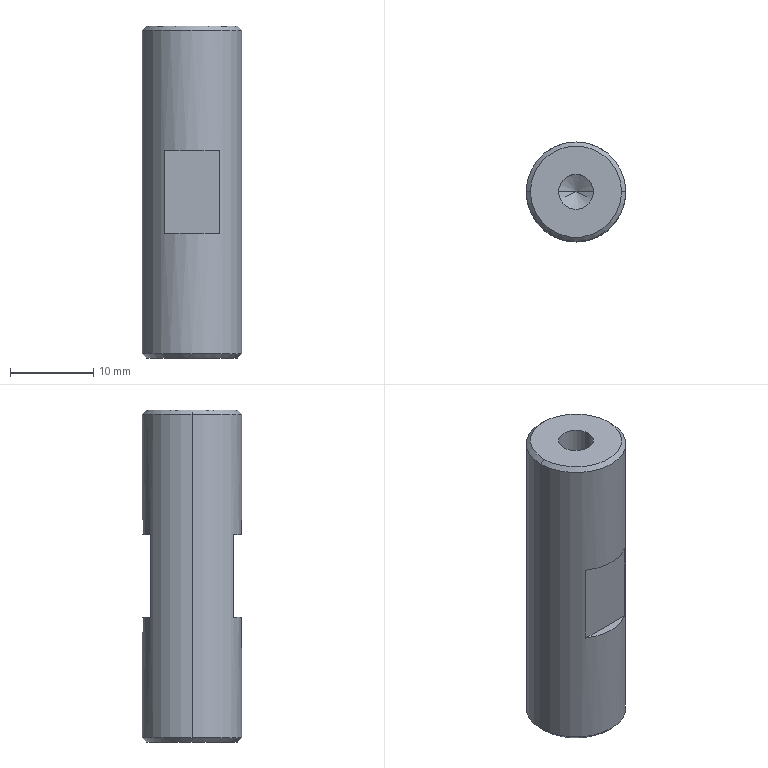Part | STEP file | QA-FC07 | 1 solid | 22 faces | box 12 x 12 x 40 mm | volume 4081 mm3 | cone 8 | plane 8 | cylinder 6 | commonest cylinder face diameters 4.2 x4 12 x2
STEP:
#1=CARTESIAN_POINT('',(0.,0.,0.));
#2=DIRECTION('',(0.,0.,1.));
#3=DIRECTION('',(1.,0.,0.));
#4=AXIS2_PLACEMENT_3D('',#1,#2,#3);
#5=CARTESIAN_POINT('',(5.5,0.,40.));
#6=VERTEX_POINT('',#5);
#7=CARTESIAN_POINT('',(-5.5,0.,40.));
#8=VERTEX_POINT('',#7);
#9=CARTESIAN_POINT('',(0.,0.,40.));
#10=DIRECTION('',(0.,0.,1.));
#11=DIRECTION('',(1.,0.,0.));
#12=AXIS2_PLACEMENT_3D('',#9,#10,#11);
#13=CIRCLE('',#12,5.5);
#14=CARTESIAN_POINT('',(0.,0.,40.));
#15=DIRECTION('',(0.,0.,-1.));
#16=DIRECTION('',(-1.,0.,0.));
#17=AXIS2_PLACEMENT_3D('',#14,#15,#16);
#18=CONICAL_SURFACE('',#17,5.5,0.7854);
#19=CARTESIAN_POINT('',(3.142,0.));
#20=DIRECTION('',(-1.,0.));
#21=VECTOR('',#20,1.);
#22=LINE('',#19,#21);
#23=(GEOMETRIC_REPRESENTATION_CONTEXT(2)PARAMETRIC_REPRESENTATION_CONTEXT()REPRESENTATION_CONTEXT('',''));
#24=DEFINITIONAL_REPRESENTATION('',(#22),#23);
#25=PCURVE('',#18,#24);
#26=CARTESIAN_POINT('',(0.,0.,40.));
#27=DIRECTION('',(0.,0.,1.));
#28=DIRECTION('',(1.,0.,0.));
#29=AXIS2_PLACEMENT_3D('',#26,#27,#28);
#30=PLANE('',#29);
#31=CARTESIAN_POINT('',(0.,0.));
#32=DIRECTION('',(1.,0.));
#33=AXIS2_PLACEMENT_2D('',#31,#32);
#34=CIRCLE('',#33,5.5);
#35=(GEOMETRIC_REPRESENTATION_CONTEXT(2)PARAMETRIC_REPRESENTATION_CONTEXT()REPRESENTATION_CONTEXT('',''));
#36=DEFINITIONAL_REPRESENTATION('',(#34),#35);
#37=PCURVE('',#30,#36);
#38=SURFACE_CURVE('',#13,(#25,#37),.PCURVE_S1.);
#39=EDGE_CURVE('',#6,#8,#38,.T.);
#40=ORIENTED_EDGE('',*,*,#39,.F.);
#41=CARTESIAN_POINT('',(6.,0.,39.5));
#42=VERTEX_POINT('',#41);
#43=CARTESIAN_POINT('',(5.5,0.,40.));
#44=DIRECTION('',(0.7071,0.,-0.7071));
#45=VECTOR('',#44,1.);
#46=LINE('',#43,#45);
#47=CARTESIAN_POINT('',(3.142,0.));
#48=DIRECTION('',(0.,1.));
#49=VECTOR('',#48,1.);
#50=LINE('',#47,#49);
#51=(GEOMETRIC_REPRESENTATION_CONTEXT(2)PARAMETRIC_REPRESENTATION_CONTEXT()REPRESENTATION_CONTEXT('',''));
#52=DEFINITIONAL_REPRESENTATION('',(#50),#51);
#53=PCURVE('',#18,#52);
#54=CARTESIAN_POINT('',(0.,0.,40.));
#55=DIRECTION('',(0.,0.,-1.));
#56=DIRECTION('',(-1.,0.,0.));
#57=AXIS2_PLACEMENT_3D('',#54,#55,#56);
#58=CONICAL_SURFACE('',#57,5.5,0.7854);
#59=CARTESIAN_POINT('',(3.142,0.));
#60=DIRECTION('',(0.,1.));
#61=VECTOR('',#60,1.);
#62=LINE('',#59,#61);
#63=(GEOMETRIC_REPRESENTATION_CONTEXT(2)PARAMETRIC_REPRESENTATION_CONTEXT()REPRESENTATION_CONTEXT('',''));
#64=DEFINITIONAL_REPRESENTATION('',(#62),#63);
#65=PCURVE('',#58,#64);
#66=SURFACE_CURVE('',#46,(#53,#65),.PCURVE_S1.);
#67=EDGE_CURVE('',#6,#42,#66,.T.);
#68=ORIENTED_EDGE('',*,*,#67,.T.);
#69=CARTESIAN_POINT('',(-6.,0.,39.5));
#70=VERTEX_POINT('',#69);
#71=CARTESIAN_POINT('',(0.,0.,39.5));
#72=DIRECTION('',(0.,0.,-1.));
#73=DIRECTION('',(1.,0.,0.));
#74=AXIS2_PLACEMENT_3D('',#71,#72,#73);
#75=CIRCLE('',#74,6.);
#76=CARTESIAN_POINT('',(-3.142,0.5));
#77=DIRECTION('',(1.,0.));
#78=VECTOR('',#77,1.);
#79=LINE('',#76,#78);
#80=(GEOMETRIC_REPRESENTATION_CONTEXT(2)PARAMETRIC_REPRESENTATION_CONTEXT()REPRESENTATION_CONTEXT('',''));
#81=DEFINITIONAL_REPRESENTATION('',(#79),#80);
#82=PCURVE('',#18,#81);
#83=CARTESIAN_POINT('',(0.,0.,40.));
#84=DIRECTION('',(0.,0.,-1.));
#85=DIRECTION('',(-1.,0.,0.));
#86=AXIS2_PLACEMENT_3D('',#83,#84,#85);
#87=CYLINDRICAL_SURFACE('',#86,6.);
#88=CARTESIAN_POINT('',(-3.142,0.5));
#89=DIRECTION('',(1.,0.));
#90=VECTOR('',#89,1.);
#91=LINE('',#88,#90);
#92=(GEOMETRIC_REPRESENTATION_CONTEXT(2)PARAMETRIC_REPRESENTATION_CONTEXT()REPRESENTATION_CONTEXT('',''));
#93=DEFINITIONAL_REPRESENTATION('',(#91),#92);
#94=PCURVE('',#87,#93);
#95=SURFACE_CURVE('',#75,(#82,#94),.PCURVE_S1.);
#96=EDGE_CURVE('',#70,#42,#95,.T.);
#97=ORIENTED_EDGE('',*,*,#96,.F.);
#98=CARTESIAN_POINT('',(-5.5,0.,40.));
#99=DIRECTION('',(-0.7071,0.,-0.7071));
#100=VECTOR('',#99,1.);
#101=LINE('',#98,#100);
#102=CARTESIAN_POINT('',(0.,0.));
#103=DIRECTION('',(0.,1.));
#104=VECTOR('',#103,1.);
#105=LINE('',#102,#104);
#106=(GEOMETRIC_REPRESENTATION_CONTEXT(2)PARAMETRIC_REPRESENTATION_CONTEXT()REPRESENTATION_CONTEXT('',''));
#107=DEFINITIONAL_REPRESENTATION('',(#105),#106);
#108=PCURVE('',#18,#107);
#109=CARTESIAN_POINT('',(6.283,0.));
#110=DIRECTION('',(0.,1.));
#111=VECTOR('',#110,1.);
#112=LINE('',#109,#111);
#113=(GEOMETRIC_REPRESENTATION_CONTEXT(2)PARAMETRIC_REPRESENTATION_CONTEXT()REPRESENTATION_CONTEXT('',''));
#114=DEFINITIONAL_REPRESENTATION('',(#112),#113);
#115=PCURVE('',#58,#114);
#116=SURFACE_CURVE('',#101,(#108,#115),.PCURVE_S1.);
#117=EDGE_CURVE('',#8,#70,#116,.T.);
#118=ORIENTED_EDGE('',*,*,#117,.F.);
#119=EDGE_LOOP('',(#40,#68,#97,#118));
#120=FACE_BOUND('',#119,.T.);
#121=ADVANCED_FACE('',(#120),#18,.T.);
#122=CARTESIAN_POINT('',(-5.5,0.,0.));
#123=VERTEX_POINT('',#122);
#124=CARTESIAN_POINT('',(5.5,0.,0.));
#125=VERTEX_POINT('',#124);
#126=CARTESIAN_POINT('',(0.,0.,0.));
#127=DIRECTION('',(0.,0.,-1.));
#128=DIRECTION('',(1.,0.,0.));
#129=AXIS2_PLACEMENT_3D('',#126,#127,#128);
#130=CIRCLE('',#129,5.5);
#131=CARTESIAN_POINT('',(0.,0.,0.5));
#132=DIRECTION('',(0.,0.,1.));
#133=DIRECTION('',(1.,0.,0.));
#134=AXIS2_PLACEMENT_3D('',#131,#132,#133);
#135=CONICAL_SURFACE('',#134,6.,0.7854);
#136=CARTESIAN_POINT('',(6.283,-0.5));
#137=DIRECTION('',(-1.,0.));
#138=VECTOR('',#137,1.);
#139=LINE('',#136,#138);
#140=(GEOMETRIC_REPRESENTATION_CONTEXT(2)PARAMETRIC_REPRESENTATION_CONTEXT()REPRESENTATION_CONTEXT('',''));
#141=DEFINITIONAL_REPRESENTATION('',(#139),#140);
#142=PCURVE('',#135,#141);
#143=CARTESIAN_POINT('',(0.,0.,0.));
#144=DIRECTION('',(0.,0.,1.));
#145=DIRECTION('',(1.,0.,0.));
#146=AXIS2_PLACEMENT_3D('',#143,#144,#145);
#147=PLANE('',#146);
#148=CARTESIAN_POINT('',(5.5,0.));
#149=CARTESIAN_POINT('',(5.5,-9.526));
#150=CARTESIAN_POINT('',(-2.75,-4.763));
#151=CARTESIAN_POINT('',(-11.,0.));
#152=CARTESIAN_POINT('',(-2.75,4.763));
#153=CARTESIAN_POINT('',(5.5,9.526));
#154=CARTESIAN_POINT('',(5.5,0.));
#155=(BOUNDED_CURVE()B_SPLINE_CURVE(2,(#148,#149,#150,#151,#152,#153,#154),.UNSPECIFIED.,.T.,.F.)B_SPLINE_CURVE_WITH_KNOTS((1,2,2,2,2,1),(-2.094,0.,2.094,4.189,6.283,8.378),.UNSPECIFIED.)CURVE()GEOMETRIC_REPRESENTATION_ITEM()RATIONAL_B_SPLINE_CURVE((1.,0.5,1.,0.5,1.,0.5,1.))REPRESENTATION_ITEM(''));
#156=(GEOMETRIC_REPRESENTATION_CONTEXT(2)PARAMETRIC_REPRESENTATION_CONTEXT()REPRESENTATION_CONTEXT('',''));
#157=DEFINITIONAL_REPRESENTATION('',(#155),#156);
#158=PCURVE('',#147,#157);
#159=SURFACE_CURVE('',#130,(#142,#158),.PCURVE_S1.);
#160=EDGE_CURVE('',#123,#125,#159,.T.);
#161=ORIENTED_EDGE('',*,*,#160,.F.);
#162=CARTESIAN_POINT('',(-6.,0.,0.5));
#163=VERTEX_POINT('',#162);
#164=CARTESIAN_POINT('',(-6.,0.,0.5));
#165=DIRECTION('',(-0.7071,0.,0.7071));
#166=VECTOR('',#165,1.);
#167=LINE('',#164,#166);
#168=CARTESIAN_POINT('',(3.142,0.));
#169=DIRECTION('',(0.,1.));
#170=VECTOR('',#169,1.);
#171=LINE('',#168,#170);
#172=(GEOMETRIC_REPRESENTATION_CONTEXT(2)PARAMETRIC_REPRESENTATION_CONTEXT()REPRESENTATION_CONTEXT('',''));
#173=DEFINITIONAL_REPRESENTATION('',(#171),#172);
#174=PCURVE('',#135,#173);
#175=CARTESIAN_POINT('',(0.,0.,0.5));
#176=DIRECTION('',(0.,0.,1.));
#177=DIRECTION('',(1.,0.,0.));
#178=AXIS2_PLACEMENT_3D('',#175,#176,#177);
#179=CONICAL_SURFACE('',#178,6.,0.7854);
#180=CARTESIAN_POINT('',(3.142,0.));
#181=DIRECTION('',(0.,1.));
#182=VECTOR('',#181,1.);
#183=LINE('',#180,#182);
#184=(GEOMETRIC_REPRESENTATION_CONTEXT(2)PARAMETRIC_REPRESENTATION_CONTEXT()REPRESENTATION_CONTEXT('',''));
#185=DEFINITIONAL_REPRESENTATION('',(#183),#184);
#186=PCURVE('',#179,#185);
#187=SURFACE_CURVE('',#167,(#174,#186),.PCURVE_S1.);
#188=EDGE_CURVE('',#123,#163,#187,.T.);
#189=ORIENTED_EDGE('',*,*,#188,.T.);
#190=CARTESIAN_POINT('',(6.,0.,0.5));
#191=VERTEX_POINT('',#190);
#192=CARTESIAN_POINT('',(0.,0.,0.5));
#193=DIRECTION('',(0.,0.,1.));
#194=DIRECTION('',(1.,0.,0.));
#195=AXIS2_PLACEMENT_3D('',#192,#193,#194);
#196=CIRCLE('',#195,6.);
#197=CARTESIAN_POINT('',(0.,0.));
#198=DIRECTION('',(1.,0.));
#199=VECTOR('',#198,1.);
#200=LINE('',#197,#199);
#201=(GEOMETRIC_REPRESENTATION_CONTEXT(2)PARAMETRIC_REPRESENTATION_CONTEXT()REPRESENTATION_CONTEXT('',''));
#202=DEFINITIONAL_REPRESENTATION('',(#200),#201);
#203=PCURVE('',#135,#202);
#204=CARTESIAN_POINT('',(3.142,39.5));
#205=DIRECTION('',(-1.,0.));
#206=VECTOR('',#205,1.);
#207=LINE('',#204,#206);
#208=(GEOMETRIC_REPRESENTATION_CONTEXT(2)PARAMETRIC_REPRESENTATION_CONTEXT()REPRESENTATION_CONTEXT('',''));
#209=DEFINITIONAL_REPRESENTATION('',(#207),#208);
#210=PCURVE('',#87,#209);
#211=SURFACE_CURVE('',#196,(#203,#210),.PCURVE_S1.);
#212=EDGE_CURVE('',#191,#163,#211,.T.);
#213=ORIENTED_EDGE('',*,*,#212,.F.);
#214=CARTESIAN_POINT('',(6.,0.,0.5));
#215=DIRECTION('',(0.7071,0.,0.7071));
#216=VECTOR('',#215,1.);
#217=LINE('',#214,#216);
#218=CARTESIAN_POINT('',(0.,0.));
#219=DIRECTION('',(0.,1.));
#220=VECTOR('',#219,1.);
#221=LINE('',#218,#220);
#222=(GEOMETRIC_REPRESENTATION_CONTEXT(2)PARAMETRIC_REPRESENTATION_CONTEXT()REPRESENTATION_CONTEXT('',''));
#223=DEFINITIONAL_REPRESENTATION('',(#221),#222);
#224=PCURVE('',#135,#223);
#225=CARTESIAN_POINT('',(6.283,0.));
#226=DIRECTION('',(0.,1.));
#227=VECTOR('',#226,1.);
#228=LINE('',#225,#227);
#229=(GEOMETRIC_REPRESENTATION_CONTEXT(2)PARAMETRIC_REPRESENTATION_CONTEXT()REPRESENTATION_CONTEXT('',''));
#230=DEFINITIONAL_REPRESENTATION('',(#228),#229);
#231=PCURVE('',#179,#230);
#232=SURFACE_CURVE('',#217,(#224,#231),.PCURVE_S1.);
#233=EDGE_CURVE('',#125,#191,#232,.T.);
#234=ORIENTED_EDGE('',*,*,#233,.F.);
#235=EDGE_LOOP('',(#161,#189,#213,#234));
#236=FACE_BOUND('',#235,.T.);
#237=ADVANCED_FACE('',(#236),#135,.T.);
#238=CARTESIAN_POINT('',(-2.1,0.,12.));
#239=VERTEX_POINT('',#238);
#240=CARTESIAN_POINT('',(-2.1,0.,0.));
#241=VERTEX_POINT('',#240);
#242=CARTESIAN_POINT('',(-2.1,0.,0.));
#243=DIRECTION('',(0.,0.,-1.));
#244=VECTOR('',#243,1.);
#245=LINE('',#242,#244);
#246=CARTESIAN_POINT('',(0.,0.,0.));
#247=DIRECTION('',(0.,0.,-1.));
#248=DIRECTION('',(-1.,0.,0.));
#249=AXIS2_PLACEMENT_3D('',#246,#247,#248);
#250=CYLINDRICAL_SURFACE('',#249,2.1);
#251=CARTESIAN_POINT('',(6.283,0.));
#252=DIRECTION('',(0.,1.));
#253=VECTOR('',#252,1.);
#254=LINE('',#251,#253);
#255=(GEOMETRIC_REPRESENTATION_CONTEXT(2)PARAMETRIC_REPRESENTATION_CONTEXT()REPRESENTATION_CONTEXT('',''));
#256=DEFINITIONAL_REPRESENTATION('',(#254),#255);
#257=PCURVE('',#250,#256);
#258=CARTESIAN_POINT('',(0.,0.,0.));
#259=DIRECTION('',(0.,0.,-1.));
#260=DIRECTION('',(-1.,0.,0.));
#261=AXIS2_PLACEMENT_3D('',#258,#259,#260);
#262=CYLINDRICAL_SURFACE('',#261,2.1);
#263=CARTESIAN_POINT('',(0.,0.));
#264=DIRECTION('',(0.,1.));
#265=VECTOR('',#264,1.);
#266=LINE('',#263,#265);
#267=(GEOMETRIC_REPRESENTATION_CONTEXT(2)PARAMETRIC_REPRESENTATION_CONTEXT()REPRESENTATION_CONTEXT('',''));
#268=DEFINITIONAL_REPRESENTATION('',(#266),#267);
#269=PCURVE('',#262,#268);
#270=SURFACE_CURVE('',#245,(#257,#269),.PCURVE_S1.);
#271=EDGE_CURVE('',#239,#241,#270,.T.);
#272=ORIENTED_EDGE('',*,*,#271,.T.);
#273=CARTESIAN_POINT('',(2.1,0.,0.));
#274=VERTEX_POINT('',#273);
#275=CARTESIAN_POINT('',(0.,0.,0.));
#276=DIRECTION('',(0.,0.,-1.));
#277=DIRECTION('',(-1.,0.,0.));
#278=AXIS2_PLACEMENT_3D('',#275,#276,#277);
#279=CIRCLE('',#278,2.1);
#280=CARTESIAN_POINT('',(0.,0.));
#281=DIRECTION('',(1.,0.));
#282=VECTOR('',#281,1.);
#283=LINE('',#280,#282);
#284=(GEOMETRIC_REPRESENTATION_CONTEXT(2)PARAMETRIC_REPRESENTATION_CONTEXT()REPRESENTATION_CONTEXT('',''));
#285=DEFINITIONAL_REPRESENTATION('',(#283),#284);
#286=PCURVE('',#250,#285);
#287=CARTESIAN_POINT('',(-2.1,0.));
#288=CARTESIAN_POINT('',(-2.1,3.637));
#289=CARTESIAN_POINT('',(1.05,1.819));
#290=CARTESIAN_POINT('',(4.2,0.));
#291=CARTESIAN_POINT('',(1.05,-1.819));
#292=CARTESIAN_POINT('',(-2.1,-3.637));
#293=CARTESIAN_POINT('',(-2.1,0.));
#294=(BOUNDED_CURVE()B_SPLINE_CURVE(2,(#287,#288,#289,#290,#291,#292,#293),.UNSPECIFIED.,.T.,.F.)B_SPLINE_CURVE_WITH_KNOTS((1,2,2,2,2,1),(-2.094,0.,2.094,4.189,6.283,8.378),.UNSPECIFIED.)CURVE()GEOMETRIC_REPRESENTATION_ITEM()RATIONAL_B_SPLINE_CURVE((1.,0.5,1.,0.5,1.,0.5,1.))REPRESENTATION_ITEM(''));
#295=(GEOMETRIC_REPRESENTATION_CONTEXT(2)PARAMETRIC_REPRESENTATION_CONTEXT()REPRESENTATION_CONTEXT('',''));
#296=DEFINITIONAL_REPRESENTATION('',(#294),#295);
#297=PCURVE('',#147,#296);
#298=SURFACE_CURVE('',#279,(#286,#297),.PCURVE_S1.);
#299=EDGE_CURVE('',#274,#241,#298,.T.);
#300=ORIENTED_EDGE('',*,*,#299,.F.);
#301=CARTESIAN_POINT('',(2.1,0.,12.));
#302=VERTEX_POINT('',#301);
#303=CARTESIAN_POINT('',(2.1,0.,0.));
#304=DIRECTION('',(0.,0.,-1.));
#305=VECTOR('',#304,1.);
#306=LINE('',#303,#305);
#307=CARTESIAN_POINT('',(3.142,0.));
#308=DIRECTION('',(0.,1.));
#309=VECTOR('',#308,1.);
#310=LINE('',#307,#309);
#311=(GEOMETRIC_REPRESENTATION_CONTEXT(2)PARAMETRIC_REPRESENTATION_CONTEXT()REPRESENTATION_CONTEXT('',''));
#312=DEFINITIONAL_REPRESENTATION('',(#310),#311);
#313=PCURVE('',#250,#312);
#314=CARTESIAN_POINT('',(3.142,0.));
#315=DIRECTION('',(0.,1.));
#316=VECTOR('',#315,1.);
#317=LINE('',#314,#316);
#318=(GEOMETRIC_REPRESENTATION_CONTEXT(2)PARAMETRIC_REPRESENTATION_CONTEXT()REPRESENTATION_CONTEXT('',''));
#319=DEFINITIONAL_REPRESENTATION('',(#317),#318);
#320=PCURVE('',#262,#319);
#321=SURFACE_CURVE('',#306,(#313,#320),.PCURVE_S1.);
#322=EDGE_CURVE('',#302,#274,#321,.T.);
#323=ORIENTED_EDGE('',*,*,#322,.F.);
#324=CARTESIAN_POINT('',(0.,0.,12.));
#325=DIRECTION('',(0.,0.,-1.));
#326=DIRECTION('',(-1.,0.,0.));
#327=AXIS2_PLACEMENT_3D('',#324,#325,#326);
#328=CIRCLE('',#327,2.1);
#329=CARTESIAN_POINT('',(0.,-12.));
#330=DIRECTION('',(1.,0.));
#331=VECTOR('',#330,1.);
#332=LINE('',#329,#331);
#333=(GEOMETRIC_REPRESENTATION_CONTEXT(2)PARAMETRIC_REPRESENTATION_CONTEXT()REPRESENTATION_CONTEXT('',''));
#334=DEFINITIONAL_REPRESENTATION('',(#332),#333);
#335=PCURVE('',#250,#334);
#336=CARTESIAN_POINT('',(0.,0.,12.));
#337=DIRECTION('',(0.,0.,-1.));
#338=DIRECTION('',(-1.,0.,0.));
#339=AXIS2_PLACEMENT_3D('',#336,#337,#338);
#340=CONICAL_SURFACE('',#339,2.1,1.03);
#341=CARTESIAN_POINT('',(0.,0.));
#342=DIRECTION('',(1.,0.));
#343=VECTOR('',#342,1.);
#344=LINE('',#341,#343);
#345=(GEOMETRIC_REPRESENTATION_CONTEXT(2)PARAMETRIC_REPRESENTATION_CONTEXT()REPRESENTATION_CONTEXT('',''));
#346=DEFINITIONAL_REPRESENTATION('',(#344),#345);
#347=PCURVE('',#340,#346);
#348=SURFACE_CURVE('',#328,(#335,#347),.PCURVE_S1.);
#349=EDGE_CURVE('',#302,#239,#348,.T.);
#350=ORIENTED_EDGE('',*,*,#349,.T.);
#351=EDGE_LOOP('',(#272,#300,#323,#350));
#352=FACE_BOUND('',#351,.F.);
#353=ADVANCED_FACE('',(#352),#250,.F.);
#354=ORIENTED_EDGE('',*,*,#349,.F.);
#355=CARTESIAN_POINT('',(0.,0.,13.262));
#356=VERTEX_POINT('',#355);
#357=CARTESIAN_POINT('',(2.1,0.,12.));
#358=DIRECTION('',(0.8572,0.,-0.515));
#359=VECTOR('',#358,1.);
#360=LINE('',#357,#359);
#361=CARTESIAN_POINT('',(3.142,0.));
#362=DIRECTION('',(0.,1.));
#363=VECTOR('',#362,1.);
#364=LINE('',#361,#363);
#365=(GEOMETRIC_REPRESENTATION_CONTEXT(2)PARAMETRIC_REPRESENTATION_CONTEXT()REPRESENTATION_CONTEXT('',''));
#366=DEFINITIONAL_REPRESENTATION('',(#364),#365);
#367=PCURVE('',#340,#366);
#368=CARTESIAN_POINT('',(0.,0.,12.));
#369=DIRECTION('',(0.,0.,-1.));
#370=DIRECTION('',(-1.,0.,0.));
#371=AXIS2_PLACEMENT_3D('',#368,#369,#370);
#372=CONICAL_SURFACE('',#371,2.1,1.03);
#373=CARTESIAN_POINT('',(3.142,0.));
#374=DIRECTION('',(0.,1.));
#375=VECTOR('',#374,1.);
#376=LINE('',#373,#375);
#377=(GEOMETRIC_REPRESENTATION_CONTEXT(2)PARAMETRIC_REPRESENTATION_CONTEXT()REPRESENTATION_CONTEXT('',''));
#378=DEFINITIONAL_REPRESENTATION('',(#376),#377);
#379=PCURVE('',#372,#378);
#380=SURFACE_CURVE('',#360,(#367,#379),.PCURVE_S1.);
#381=EDGE_CURVE('',#356,#302,#380,.T.);
#382=ORIENTED_EDGE('',*,*,#381,.F.);
#383=CARTESIAN_POINT('',(-2.1,0.,12.));
#384=DIRECTION('',(-0.8572,0.,-0.515));
#385=VECTOR('',#384,1.);
#386=LINE('',#383,#385);
#387=CARTESIAN_POINT('',(6.283,0.));
#388=DIRECTION('',(0.,1.));
#389=VECTOR('',#388,1.);
#390=LINE('',#387,#389);
#391=(GEOMETRIC_REPRESENTATION_CONTEXT(2)PARAMETRIC_REPRESENTATION_CONTEXT()REPRESENTATION_CONTEXT('',''));
#392=DEFINITIONAL_REPRESENTATION('',(#390),#391);
#393=PCURVE('',#340,#392);
#394=CARTESIAN_POINT('',(0.,0.));
#395=DIRECTION('',(0.,1.));
#396=VECTOR('',#395,1.);
#397=LINE('',#394,#396);
#398=(GEOMETRIC_REPRESENTATION_CONTEXT(2)PARAMETRIC_REPRESENTATION_CONTEXT()REPRESENTATION_CONTEXT('',''));
#399=DEFINITIONAL_REPRESENTATION('',(#397),#398);
#400=PCURVE('',#372,#399);
#401=SURFACE_CURVE('',#386,(#393,#400),.PCURVE_S1.);
#402=EDGE_CURVE('',#356,#239,#401,.T.);
#403=ORIENTED_EDGE('',*,*,#402,.T.);
#404=EDGE_LOOP('',(#354,#382,#403));
#405=FACE_BOUND('',#404,.F.);
#406=ADVANCED_FACE('',(#405),#340,.F.);
#407=CARTESIAN_POINT('',(2.1,0.,28.));
#408=VERTEX_POINT('',#407);
#409=CARTESIAN_POINT('',(2.1,0.,40.));
#410=VERTEX_POINT('',#409);
#411=CARTESIAN_POINT('',(2.1,0.,40.));
#412=DIRECTION('',(0.,0.,1.));
#413=VECTOR('',#412,1.);
#414=LINE('',#411,#413);
#415=CARTESIAN_POINT('',(0.,0.,40.));
#416=DIRECTION('',(0.,0.,1.));
#417=DIRECTION('',(1.,0.,0.));
#418=AXIS2_PLACEMENT_3D('',#415,#416,#417);
#419=CYLINDRICAL_SURFACE('',#418,2.1);
#420=CARTESIAN_POINT('',(6.283,0.));
#421=DIRECTION('',(0.,1.));
#422=VECTOR('',#421,1.);
#423=LINE('',#420,#422);
#424=(GEOMETRIC_REPRESENTATION_CONTEXT(2)PARAMETRIC_REPRESENTATION_CONTEXT()REPRESENTATION_CONTEXT('',''));
#425=DEFINITIONAL_REPRESENTATION('',(#423),#424);
#426=PCURVE('',#419,#425);
#427=CARTESIAN_POINT('',(0.,0.,40.));
#428=DIRECTION('',(0.,0.,1.));
#429=DIRECTION('',(1.,0.,0.));
#430=AXIS2_PLACEMENT_3D('',#427,#428,#429);
#431=CYLINDRICAL_SURFACE('',#430,2.1);
#432=CARTESIAN_POINT('',(0.,0.));
#433=DIRECTION('',(0.,1.));
#434=VECTOR('',#433,1.);
#435=LINE('',#432,#434);
#436=(GEOMETRIC_REPRESENTATION_CONTEXT(2)PARAMETRIC_REPRESENTATION_CONTEXT()REPRESENTATION_CONTEXT('',''));
#437=DEFINITIONAL_REPRESENTATION('',(#435),#436);
#438=PCURVE('',#431,#437);
#439=SURFACE_CURVE('',#414,(#426,#438),.PCURVE_S1.);
#440=EDGE_CURVE('',#408,#410,#439,.T.);
#441=ORIENTED_EDGE('',*,*,#440,.T.);
#442=CARTESIAN_POINT('',(-2.1,0.,40.));
#443=VERTEX_POINT('',#442);
#444=CARTESIAN_POINT('',(0.,0.,40.));
#445=DIRECTION('',(0.,0.,1.));
#446=DIRECTION('',(1.,0.,0.));
#447=AXIS2_PLACEMENT_3D('',#444,#445,#446);
#448=CIRCLE('',#447,2.1);
#449=CARTESIAN_POINT('',(0.,0.));
#450=DIRECTION('',(1.,0.));
#451=VECTOR('',#450,1.);
#452=LINE('',#449,#451);
#453=(GEOMETRIC_REPRESENTATION_CONTEXT(2)PARAMETRIC_REPRESENTATION_CONTEXT()REPRESENTATION_CONTEXT('',''));
#454=DEFINITIONAL_REPRESENTATION('',(#452),#453);
#455=PCURVE('',#419,#454);
#456=CARTESIAN_POINT('',(0.,0.));
#457=DIRECTION('',(1.,0.));
#458=AXIS2_PLACEMENT_2D('',#456,#457);
#459=CIRCLE('',#458,2.1);
#460=(GEOMETRIC_REPRESENTATION_CONTEXT(2)PARAMETRIC_REPRESENTATION_CONTEXT()REPRESENTATION_CONTEXT('',''));
#461=DEFINITIONAL_REPRESENTATION('',(#459),#460);
#462=PCURVE('',#30,#461);
#463=SURFACE_CURVE('',#448,(#455,#462),.PCURVE_S1.);
#464=EDGE_CURVE('',#443,#410,#463,.T.);
#465=ORIENTED_EDGE('',*,*,#464,.F.);
#466=CARTESIAN_POINT('',(-2.1,0.,28.));
#467=VERTEX_POINT('',#466);
#468=CARTESIAN_POINT('',(-2.1,0.,40.));
#469=DIRECTION('',(0.,0.,1.));
#470=VECTOR('',#469,1.);
#471=LINE('',#468,#470);
#472=CARTESIAN_POINT('',(3.142,0.));
#473=DIRECTION('',(0.,1.));
#474=VECTOR('',#473,1.);
#475=LINE('',#472,#474);
#476=(GEOMETRIC_REPRESENTATION_CONTEXT(2)PARAMETRIC_REPRESENTATION_CONTEXT()REPRESENTATION_CONTEXT('',''));
#477=DEFINITIONAL_REPRESENTATION('',(#475),#476);
#478=PCURVE('',#419,#477);
#479=CARTESIAN_POINT('',(3.142,0.));
#480=DIRECTION('',(0.,1.));
#481=VECTOR('',#480,1.);
#482=LINE('',#479,#481);
#483=(GEOMETRIC_REPRESENTATION_CONTEXT(2)PARAMETRIC_REPRESENTATION_CONTEXT()REPRESENTATION_CONTEXT('',''));
#484=DEFINITIONAL_REPRESENTATION('',(#482),#483);
#485=PCURVE('',#431,#484);
#486=SURFACE_CURVE('',#471,(#478,#485),.PCURVE_S1.);
#487=EDGE_CURVE('',#467,#443,#486,.T.);
#488=ORIENTED_EDGE('',*,*,#487,.F.);
#489=CARTESIAN_POINT('',(0.,0.,28.));
#490=DIRECTION('',(0.,0.,1.));
#491=DIRECTION('',(1.,0.,0.));
#492=AXIS2_PLACEMENT_3D('',#489,#490,#491);
#493=CIRCLE('',#492,2.1);
#494=CARTESIAN_POINT('',(0.,-12.));
#495=DIRECTION('',(1.,0.));
#496=VECTOR('',#495,1.);
#497=LINE('',#494,#496);
#498=(GEOMETRIC_REPRESENTATION_CONTEXT(2)PARAMETRIC_REPRESENTATION_CONTEXT()REPRESENTATION_CONTEXT('',''));
#499=DEFINITIONAL_REPRESENTATION('',(#497),#498);
#500=PCURVE('',#419,#499);
#501=CARTESIAN_POINT('',(0.,0.,28.));
#502=DIRECTION('',(0.,0.,1.));
#503=DIRECTION('',(1.,0.,0.));
#504=AXIS2_PLACEMENT_3D('',#501,#502,#503);
#505=CONICAL_SURFACE('',#504,2.1,1.03);
#506=CARTESIAN_POINT('',(0.,0.));
#507=DIRECTION('',(1.,0.));
#508=VECTOR('',#507,1.);
#509=LINE('',#506,#508);
#510=(GEOMETRIC_REPRESENTATION_CONTEXT(2)PARAMETRIC_REPRESENTATION_CONTEXT()REPRESENTATION_CONTEXT('',''));
#511=DEFINITIONAL_REPRESENTATION('',(#509),#510);
#512=PCURVE('',#505,#511);
#513=SURFACE_CURVE('',#493,(#500,#512),.PCURVE_S1.);
#514=EDGE_CURVE('',#467,#408,#513,.T.);
#515=ORIENTED_EDGE('',*,*,#514,.T.);
#516=EDGE_LOOP('',(#441,#465,#488,#515));
#517=FACE_BOUND('',#516,.F.);
#518=ADVANCED_FACE('',(#517),#419,.F.);
#519=ORIENTED_EDGE('',*,*,#514,.F.);
#520=CARTESIAN_POINT('',(0.,0.,26.738));
#521=VERTEX_POINT('',#520);
#522=CARTESIAN_POINT('',(-2.1,0.,28.));
#523=DIRECTION('',(-0.8572,0.,0.515));
#524=VECTOR('',#523,1.);
#525=LINE('',#522,#524);
#526=CARTESIAN_POINT('',(3.142,0.));
#527=DIRECTION('',(0.,1.));
#528=VECTOR('',#527,1.);
#529=LINE('',#526,#528);
#530=(GEOMETRIC_REPRESENTATION_CONTEXT(2)PARAMETRIC_REPRESENTATION_CONTEXT()REPRESENTATION_CONTEXT('',''));
#531=DEFINITIONAL_REPRESENTATION('',(#529),#530);
#532=PCURVE('',#505,#531);
#533=CARTESIAN_POINT('',(0.,0.,28.));
#534=DIRECTION('',(0.,0.,1.));
#535=DIRECTION('',(1.,0.,0.));
#536=AXIS2_PLACEMENT_3D('',#533,#534,#535);
#537=CONICAL_SURFACE('',#536,2.1,1.03);
#538=CARTESIAN_POINT('',(3.142,0.));
#539=DIRECTION('',(0.,1.));
#540=VECTOR('',#539,1.);
#541=LINE('',#538,#540);
#542=(GEOMETRIC_REPRESENTATION_CONTEXT(2)PARAMETRIC_REPRESENTATION_CONTEXT()REPRESENTATION_CONTEXT('',''));
#543=DEFINITIONAL_REPRESENTATION('',(#541),#542);
#544=PCURVE('',#537,#543);
#545=SURFACE_CURVE('',#525,(#532,#544),.PCURVE_S1.);
#546=EDGE_CURVE('',#521,#467,#545,.T.);
#547=ORIENTED_EDGE('',*,*,#546,.F.);
#548=CARTESIAN_POINT('',(2.1,0.,28.));
#549=DIRECTION('',(0.8572,0.,0.515));
#550=VECTOR('',#549,1.);
#551=LINE('',#548,#550);
#552=CARTESIAN_POINT('',(6.283,0.));
#553=DIRECTION('',(0.,1.));
#554=VECTOR('',#553,1.);
#555=LINE('',#552,#554);
#556=(GEOMETRIC_REPRESENTATION_CONTEXT(2)PARAMETRIC_REPRESENTATION_CONTEXT()REPRESENTATION_CONTEXT('',''));
#557=DEFINITIONAL_REPRESENTATION('',(#555),#556);
#558=PCURVE('',#505,#557);
#559=CARTESIAN_POINT('',(0.,0.));
#560=DIRECTION('',(0.,1.));
#561=VECTOR('',#560,1.);
#562=LINE('',#559,#561);
#563=(GEOMETRIC_REPRESENTATION_CONTEXT(2)PARAMETRIC_REPRESENTATION_CONTEXT()REPRESENTATION_CONTEXT('',''));
#564=DEFINITIONAL_REPRESENTATION('',(#562),#563);
#565=PCURVE('',#537,#564);
#566=SURFACE_CURVE('',#551,(#558,#565),.PCURVE_S1.);
#567=EDGE_CURVE('',#521,#408,#566,.T.);
#568=ORIENTED_EDGE('',*,*,#567,.T.);
#569=EDGE_LOOP('',(#519,#547,#568));
#570=FACE_BOUND('',#569,.F.);
#571=ADVANCED_FACE('',(#570),#505,.F.);
#572=CARTESIAN_POINT('',(-3.317,5.,15.));
#573=VERTEX_POINT('',#572);
#574=CARTESIAN_POINT('',(-3.317,5.,25.));
#575=VERTEX_POINT('',#574);
#576=CARTESIAN_POINT('',(-3.317,5.,40.));
#577=DIRECTION('',(0.,0.,1.));
#578=VECTOR('',#577,1.);
#579=LINE('',#576,#578);
#580=CARTESIAN_POINT('',(0.9851,0.));
#581=DIRECTION('',(0.,-1.));
#582=VECTOR('',#581,1.);
#583=LINE('',#580,#582);
#584=(GEOMETRIC_REPRESENTATION_CONTEXT(2)PARAMETRIC_REPRESENTATION_CONTEXT()REPRESENTATION_CONTEXT('',''));
#585=DEFINITIONAL_REPRESENTATION('',(#583),#584);
#586=PCURVE('',#87,#585);
#587=CARTESIAN_POINT('',(0.,5.,0.));
#588=DIRECTION('',(0.,1.,0.));
#589=DIRECTION('',(0.,0.,1.));
#590=AXIS2_PLACEMENT_3D('',#587,#588,#589);
#591=PLANE('',#590);
#592=CARTESIAN_POINT('',(40.,-3.317));
#593=DIRECTION('',(1.,0.));
#594=VECTOR('',#593,1.);
#595=LINE('',#592,#594);
#596=(GEOMETRIC_REPRESENTATION_CONTEXT(2)PARAMETRIC_REPRESENTATION_CONTEXT()REPRESENTATION_CONTEXT('',''));
#597=DEFINITIONAL_REPRESENTATION('',(#595),#596);
#598=PCURVE('',#591,#597);
#599=SURFACE_CURVE('',#579,(#586,#598),.PCURVE_S1.);
#600=EDGE_CURVE('',#573,#575,#599,.T.);
#601=ORIENTED_EDGE('',*,*,#600,.F.);
#602=CARTESIAN_POINT('',(3.317,5.,15.));
#603=VERTEX_POINT('',#602);
#604=CARTESIAN_POINT('',(0.,0.,15.));
#605=DIRECTION('',(0.,0.,-1.));
#606=DIRECTION('',(-1.,0.,0.));
#607=AXIS2_PLACEMENT_3D('',#604,#605,#606);
#608=CIRCLE('',#607,6.);
#609=CARTESIAN_POINT('',(0.,25.));
#610=DIRECTION('',(1.,0.));
#611=VECTOR('',#610,1.);
#612=LINE('',#609,#611);
#613=(GEOMETRIC_REPRESENTATION_CONTEXT(2)PARAMETRIC_REPRESENTATION_CONTEXT()REPRESENTATION_CONTEXT('',''));
#614=DEFINITIONAL_REPRESENTATION('',(#612),#613);
#615=PCURVE('',#87,#614);
#616=CARTESIAN_POINT('',(-10.,5.,15.));
#617=DIRECTION('',(0.,0.,-1.));
#618=DIRECTION('',(-1.,0.,0.));
#619=AXIS2_PLACEMENT_3D('',#616,#617,#618);
#620=PLANE('',#619);
#621=CARTESIAN_POINT('',(-10.,-5.));
#622=DIRECTION('',(1.,0.));
#623=AXIS2_PLACEMENT_2D('',#621,#622);
#624=CIRCLE('',#623,6.);
#625=(GEOMETRIC_REPRESENTATION_CONTEXT(2)PARAMETRIC_REPRESENTATION_CONTEXT()REPRESENTATION_CONTEXT('',''));
#626=DEFINITIONAL_REPRESENTATION('',(#624),#625);
#627=PCURVE('',#620,#626);
#628=SURFACE_CURVE('',#608,(#615,#627),.PCURVE_S1.);
#629=EDGE_CURVE('',#573,#603,#628,.T.);
#630=ORIENTED_EDGE('',*,*,#629,.T.);
#631=CARTESIAN_POINT('',(3.317,5.,25.));
#632=VERTEX_POINT('',#631);
#633=CARTESIAN_POINT('',(3.317,5.,40.));
#634=DIRECTION('',(0.,0.,-1.));
#635=VECTOR('',#634,1.);
#636=LINE('',#633,#635);
#637=CARTESIAN_POINT('',(2.156,0.));
#638=DIRECTION('',(0.,1.));
#639=VECTOR('',#638,1.);
#640=LINE('',#637,#639);
#641=(GEOMETRIC_REPRESENTATION_CONTEXT(2)PARAMETRIC_REPRESENTATION_CONTEXT()REPRESENTATION_CONTEXT('',''));
#642=DEFINITIONAL_REPRESENTATION('',(#640),#641);
#643=PCURVE('',#87,#642);
#644=CARTESIAN_POINT('',(40.,3.317));
#645=DIRECTION('',(-1.,0.));
#646=VECTOR('',#645,1.);
#647=LINE('',#644,#646);
#648=(GEOMETRIC_REPRESENTATION_CONTEXT(2)PARAMETRIC_REPRESENTATION_CONTEXT()REPRESENTATION_CONTEXT('',''));
#649=DEFINITIONAL_REPRESENTATION('',(#647),#648);
#650=PCURVE('',#591,#649);
#651=SURFACE_CURVE('',#636,(#643,#650),.PCURVE_S1.);
#652=EDGE_CURVE('',#632,#603,#651,.T.);
#653=ORIENTED_EDGE('',*,*,#652,.F.);
#654=CARTESIAN_POINT('',(0.,0.,25.));
#655=DIRECTION('',(0.,0.,1.));
#656=DIRECTION('',(1.,0.,0.));
#657=AXIS2_PLACEMENT_3D('',#654,#655,#656);
#658=CIRCLE('',#657,6.);
#659=CARTESIAN_POINT('',(3.142,15.));
#660=DIRECTION('',(-1.,0.));
#661=VECTOR('',#660,1.);
#662=LINE('',#659,#661);
#663=(GEOMETRIC_REPRESENTATION_CONTEXT(2)PARAMETRIC_REPRESENTATION_CONTEXT()REPRESENTATION_CONTEXT('',''));
#664=DEFINITIONAL_REPRESENTATION('',(#662),#663);
#665=PCURVE('',#87,#664);
#666=CARTESIAN_POINT('',(-10.,5.,25.));
#667=DIRECTION('',(0.,0.,1.));
#668=DIRECTION('',(1.,0.,0.));
#669=AXIS2_PLACEMENT_3D('',#666,#667,#668);
#670=PLANE('',#669);
#671=CARTESIAN_POINT('',(10.,-5.));
#672=DIRECTION('',(1.,0.));
#673=AXIS2_PLACEMENT_2D('',#671,#672);
#674=CIRCLE('',#673,6.);
#675=(GEOMETRIC_REPRESENTATION_CONTEXT(2)PARAMETRIC_REPRESENTATION_CONTEXT()REPRESENTATION_CONTEXT('',''));
#676=DEFINITIONAL_REPRESENTATION('',(#674),#675);
#677=PCURVE('',#670,#676);
#678=SURFACE_CURVE('',#658,(#665,#677),.PCURVE_S1.);
#679=EDGE_CURVE('',#632,#575,#678,.T.);
#680=ORIENTED_EDGE('',*,*,#679,.T.);
#681=EDGE_LOOP('',(#601,#630,#653,#680));
#682=FACE_BOUND('',#681,.T.);
#683=ORIENTED_EDGE('',*,*,#96,.T.);
#684=CARTESIAN_POINT('',(6.,0.,40.));
#685=DIRECTION('',(0.,0.,-1.));
#686=VECTOR('',#685,1.);
#687=LINE('',#684,#686);
#688=CARTESIAN_POINT('',(3.142,0.));
#689=DIRECTION('',(0.,1.));
#690=VECTOR('',#689,1.);
#691=LINE('',#688,#690);
#692=(GEOMETRIC_REPRESENTATION_CONTEXT(2)PARAMETRIC_REPRESENTATION_CONTEXT()REPRESENTATION_CONTEXT('',''));
#693=DEFINITIONAL_REPRESENTATION('',(#691),#692);
#694=PCURVE('',#87,#693);
#695=CARTESIAN_POINT('',(0.,0.,40.));
#696=DIRECTION('',(0.,0.,-1.));
#697=DIRECTION('',(-1.,0.,0.));
#698=AXIS2_PLACEMENT_3D('',#695,#696,#697);
#699=CYLINDRICAL_SURFACE('',#698,6.);
#700=CARTESIAN_POINT('',(3.142,0.));
#701=DIRECTION('',(0.,1.));
#702=VECTOR('',#701,1.);
#703=LINE('',#700,#702);
#704=(GEOMETRIC_REPRESENTATION_CONTEXT(2)PARAMETRIC_REPRESENTATION_CONTEXT()REPRESENTATION_CONTEXT('',''));
#705=DEFINITIONAL_REPRESENTATION('',(#703),#704);
#706=PCURVE('',#699,#705);
#707=SURFACE_CURVE('',#687,(#694,#706),.PCURVE_S1.);
#708=EDGE_CURVE('',#42,#191,#707,.T.);
#709=ORIENTED_EDGE('',*,*,#708,.T.);
#710=ORIENTED_EDGE('',*,*,#212,.T.);
#711=CARTESIAN_POINT('',(-6.,0.,40.));
#712=DIRECTION('',(0.,0.,-1.));
#713=VECTOR('',#712,1.);
#714=LINE('',#711,#713);
#715=CARTESIAN_POINT('',(0.,0.));
#716=DIRECTION('',(0.,1.));
#717=VECTOR('',#716,1.);
#718=LINE('',#715,#717);
#719=(GEOMETRIC_REPRESENTATION_CONTEXT(2)PARAMETRIC_REPRESENTATION_CONTEXT()REPRESENTATION_CONTEXT('',''));
#720=DEFINITIONAL_REPRESENTATION('',(#718),#719);
#721=PCURVE('',#87,#720);
#722=CARTESIAN_POINT('',(6.283,0.));
#723=DIRECTION('',(0.,1.));
#724=VECTOR('',#723,1.);
#725=LINE('',#722,#724);
#726=(GEOMETRIC_REPRESENTATION_CONTEXT(2)PARAMETRIC_REPRESENTATION_CONTEXT()REPRESENTATION_CONTEXT('',''));
#727=DEFINITIONAL_REPRESENTATION('',(#725),#726);
#728=PCURVE('',#699,#727);
#729=SURFACE_CURVE('',#714,(#721,#728),.PCURVE_S1.);
#730=EDGE_CURVE('',#70,#163,#729,.T.);
#731=ORIENTED_EDGE('',*,*,#730,.F.);
#732=EDGE_LOOP('',(#683,#709,#710,#731));
#733=FACE_BOUND('',#732,.T.);
#734=ADVANCED_FACE('',(#682,#733),#87,.T.);
#735=ORIENTED_EDGE('',*,*,#708,.F.);
#736=CARTESIAN_POINT('',(0.,0.,39.5));
#737=DIRECTION('',(0.,0.,-1.));
#738=DIRECTION('',(1.,0.,0.));
#739=AXIS2_PLACEMENT_3D('',#736,#737,#738);
#740=CIRCLE('',#739,6.);
#741=CARTESIAN_POINT('',(3.142,0.5));
#742=DIRECTION('',(1.,0.));
#743=VECTOR('',#742,1.);
#744=LINE('',#741,#743);
#745=(GEOMETRIC_REPRESENTATION_CONTEXT(2)PARAMETRIC_REPRESENTATION_CONTEXT()REPRESENTATION_CONTEXT('',''));
#746=DEFINITIONAL_REPRESENTATION('',(#744),#745);
#747=PCURVE('',#699,#746);
#748=CARTESIAN_POINT('',(3.142,0.5));
#749=DIRECTION('',(1.,0.));
#750=VECTOR('',#749,1.);
#751=LINE('',#748,#750);
#752=(GEOMETRIC_REPRESENTATION_CONTEXT(2)PARAMETRIC_REPRESENTATION_CONTEXT()REPRESENTATION_CONTEXT('',''));
#753=DEFINITIONAL_REPRESENTATION('',(#751),#752);
#754=PCURVE('',#58,#753);
#755=SURFACE_CURVE('',#740,(#747,#754),.PCURVE_S1.);
#756=EDGE_CURVE('',#42,#70,#755,.T.);
#757=ORIENTED_EDGE('',*,*,#756,.T.);
#758=ORIENTED_EDGE('',*,*,#730,.T.);
#759=CARTESIAN_POINT('',(0.,0.,0.5));
#760=DIRECTION('',(0.,0.,1.));
#761=DIRECTION('',(1.,0.,0.));
#762=AXIS2_PLACEMENT_3D('',#759,#760,#761);
#763=CIRCLE('',#762,6.);
#764=CARTESIAN_POINT('',(9.425,39.5));
#765=DIRECTION('',(-1.,0.));
#766=VECTOR('',#765,1.);
#767=LINE('',#764,#766);
#768=(GEOMETRIC_REPRESENTATION_CONTEXT(2)PARAMETRIC_REPRESENTATION_CONTEXT()REPRESENTATION_CONTEXT('',''));
#769=DEFINITIONAL_REPRESENTATION('',(#767),#768);
#770=PCURVE('',#699,#769);
#771=CARTESIAN_POINT('',(0.,0.));
#772=DIRECTION('',(1.,0.));
#773=VECTOR('',#772,1.);
#774=LINE('',#771,#773);
#775=(GEOMETRIC_REPRESENTATION_CONTEXT(2)PARAMETRIC_REPRESENTATION_CONTEXT()REPRESENTATION_CONTEXT('',''));
#776=DEFINITIONAL_REPRESENTATION('',(#774),#775);
#777=PCURVE('',#179,#776);
#778=SURFACE_CURVE('',#763,(#770,#777),.PCURVE_S1.);
#779=EDGE_CURVE('',#163,#191,#778,.T.);
#780=ORIENTED_EDGE('',*,*,#779,.T.);
#781=EDGE_LOOP('',(#735,#757,#758,#780));
#782=FACE_BOUND('',#781,.T.);
#783=CARTESIAN_POINT('',(3.317,-5.,15.));
#784=VERTEX_POINT('',#783);
#785=CARTESIAN_POINT('',(3.317,-5.,25.));
#786=VERTEX_POINT('',#785);
#787=CARTESIAN_POINT('',(3.317,-5.,40.));
#788=DIRECTION('',(0.,0.,1.));
#789=VECTOR('',#788,1.);
#790=LINE('',#787,#789);
#791=CARTESIAN_POINT('',(4.127,0.));
#792=DIRECTION('',(0.,-1.));
#793=VECTOR('',#792,1.);
#794=LINE('',#791,#793);
#795=(GEOMETRIC_REPRESENTATION_CONTEXT(2)PARAMETRIC_REPRESENTATION_CONTEXT()REPRESENTATION_CONTEXT('',''));
#796=DEFINITIONAL_REPRESENTATION('',(#794),#795);
#797=PCURVE('',#699,#796);
#798=CARTESIAN_POINT('',(0.,-5.,0.));
#799=DIRECTION('',(0.,-1.,0.));
#800=DIRECTION('',(0.,0.,1.));
#801=AXIS2_PLACEMENT_3D('',#798,#799,#800);
#802=PLANE('',#801);
#803=CARTESIAN_POINT('',(40.,-3.317));
#804=DIRECTION('',(1.,0.));
#805=VECTOR('',#804,1.);
#806=LINE('',#803,#805);
#807=(GEOMETRIC_REPRESENTATION_CONTEXT(2)PARAMETRIC_REPRESENTATION_CONTEXT()REPRESENTATION_CONTEXT('',''));
#808=DEFINITIONAL_REPRESENTATION('',(#806),#807);
#809=PCURVE('',#802,#808);
#810=SURFACE_CURVE('',#790,(#797,#809),.PCURVE_S1.);
#811=EDGE_CURVE('',#784,#786,#810,.T.);
#812=ORIENTED_EDGE('',*,*,#811,.F.);
#813=CARTESIAN_POINT('',(-3.317,-5.,15.));
#814=VERTEX_POINT('',#813);
#815=CARTESIAN_POINT('',(0.,0.,15.));
#816=DIRECTION('',(0.,0.,-1.));
#817=DIRECTION('',(-1.,0.,0.));
#818=AXIS2_PLACEMENT_3D('',#815,#816,#817);
#819=CIRCLE('',#818,6.);
#820=CARTESIAN_POINT('',(0.,25.));
#821=DIRECTION('',(1.,0.));
#822=VECTOR('',#821,1.);
#823=LINE('',#820,#822);
#824=(GEOMETRIC_REPRESENTATION_CONTEXT(2)PARAMETRIC_REPRESENTATION_CONTEXT()REPRESENTATION_CONTEXT('',''));
#825=DEFINITIONAL_REPRESENTATION('',(#823),#824);
#826=PCURVE('',#699,#825);
#827=CARTESIAN_POINT('',(10.,-5.,15.));
#828=DIRECTION('',(0.,0.,-1.));
#829=DIRECTION('',(-1.,0.,0.));
#830=AXIS2_PLACEMENT_3D('',#827,#828,#829);
#831=PLANE('',#830);
#832=CARTESIAN_POINT('',(10.,5.));
#833=DIRECTION('',(1.,0.));
#834=AXIS2_PLACEMENT_2D('',#832,#833);
#835=CIRCLE('',#834,6.);
#836=(GEOMETRIC_REPRESENTATION_CONTEXT(2)PARAMETRIC_REPRESENTATION_CONTEXT()REPRESENTATION_CONTEXT('',''));
#837=DEFINITIONAL_REPRESENTATION('',(#835),#836);
#838=PCURVE('',#831,#837);
#839=SURFACE_CURVE('',#819,(#826,#838),.PCURVE_S1.);
#840=EDGE_CURVE('',#784,#814,#839,.T.);
#841=ORIENTED_EDGE('',*,*,#840,.T.);
#842=CARTESIAN_POINT('',(-3.317,-5.,25.));
#843=VERTEX_POINT('',#842);
#844=CARTESIAN_POINT('',(-3.317,-5.,40.));
#845=DIRECTION('',(0.,0.,-1.));
#846=VECTOR('',#845,1.);
#847=LINE('',#844,#846);
#848=CARTESIAN_POINT('',(5.298,0.));
#849=DIRECTION('',(0.,1.));
#850=VECTOR('',#849,1.);
#851=LINE('',#848,#850);
#852=(GEOMETRIC_REPRESENTATION_CONTEXT(2)PARAMETRIC_REPRESENTATION_CONTEXT()REPRESENTATION_CONTEXT('',''));
#853=DEFINITIONAL_REPRESENTATION('',(#851),#852);
#854=PCURVE('',#699,#853);
#855=CARTESIAN_POINT('',(40.,3.317));
#856=DIRECTION('',(-1.,0.));
#857=VECTOR('',#856,1.);
#858=LINE('',#855,#857);
#859=(GEOMETRIC_REPRESENTATION_CONTEXT(2)PARAMETRIC_REPRESENTATION_CONTEXT()REPRESENTATION_CONTEXT('',''));
#860=DEFINITIONAL_REPRESENTATION('',(#858),#859);
#861=PCURVE('',#802,#860);
#862=SURFACE_CURVE('',#847,(#854,#861),.PCURVE_S1.);
#863=EDGE_CURVE('',#843,#814,#862,.T.);
#864=ORIENTED_EDGE('',*,*,#863,.F.);
#865=CARTESIAN_POINT('',(0.,0.,25.));
#866=DIRECTION('',(0.,0.,1.));
#867=DIRECTION('',(1.,0.,0.));
#868=AXIS2_PLACEMENT_3D('',#865,#866,#867);
#869=CIRCLE('',#868,6.);
#870=CARTESIAN_POINT('',(9.425,15.));
#871=DIRECTION('',(-1.,0.));
#872=VECTOR('',#871,1.);
#873=LINE('',#870,#872);
#874=(GEOMETRIC_REPRESENTATION_CONTEXT(2)PARAMETRIC_REPRESENTATION_CONTEXT()REPRESENTATION_CONTEXT('',''));
#875=DEFINITIONAL_REPRESENTATION('',(#873),#874);
#876=PCURVE('',#699,#875);
#877=CARTESIAN_POINT('',(10.,-5.,25.));
#878=DIRECTION('',(0.,0.,1.));
#879=DIRECTION('',(1.,0.,0.));
#880=AXIS2_PLACEMENT_3D('',#877,#878,#879);
#881=PLANE('',#880);
#882=CARTESIAN_POINT('',(-10.,5.));
#883=DIRECTION('',(1.,0.));
#884=AXIS2_PLACEMENT_2D('',#882,#883);
#885=CIRCLE('',#884,6.);
#886=(GEOMETRIC_REPRESENTATION_CONTEXT(2)PARAMETRIC_REPRESENTATION_CONTEXT()REPRESENTATION_CONTEXT('',''));
#887=DEFINITIONAL_REPRESENTATION('',(#885),#886);
#888=PCURVE('',#881,#887);
#889=SURFACE_CURVE('',#869,(#876,#888),.PCURVE_S1.);
#890=EDGE_CURVE('',#843,#786,#889,.T.);
#891=ORIENTED_EDGE('',*,*,#890,.T.);
#892=EDGE_LOOP('',(#812,#841,#864,#891));
#893=FACE_BOUND('',#892,.T.);
#894=ADVANCED_FACE('',(#782,#893),#699,.T.);
#895=CARTESIAN_POINT('',(0.,0.,40.));
#896=DIRECTION('',(0.,0.,1.));
#897=DIRECTION('',(1.,0.,0.));
#898=AXIS2_PLACEMENT_3D('',#895,#896,#897);
#899=CIRCLE('',#898,5.5);
#900=CARTESIAN_POINT('',(0.,0.));
#901=DIRECTION('',(1.,0.));
#902=AXIS2_PLACEMENT_2D('',#900,#901);
#903=CIRCLE('',#902,5.5);
#904=(GEOMETRIC_REPRESENTATION_CONTEXT(2)PARAMETRIC_REPRESENTATION_CONTEXT()REPRESENTATION_CONTEXT('',''));
#905=DEFINITIONAL_REPRESENTATION('',(#903),#904);
#906=PCURVE('',#30,#905);
#907=CARTESIAN_POINT('',(9.425,0.));
#908=DIRECTION('',(-1.,0.));
#909=VECTOR('',#908,1.);
#910=LINE('',#907,#909);
#911=(GEOMETRIC_REPRESENTATION_CONTEXT(2)PARAMETRIC_REPRESENTATION_CONTEXT()REPRESENTATION_CONTEXT('',''));
#912=DEFINITIONAL_REPRESENTATION('',(#910),#911);
#913=PCURVE('',#58,#912);
#914=SURFACE_CURVE('',#899,(#906,#913),.PCURVE_S1.);
#915=EDGE_CURVE('',#8,#6,#914,.T.);
#916=ORIENTED_EDGE('',*,*,#915,.T.);
#917=ORIENTED_EDGE('',*,*,#39,.T.);
#918=EDGE_LOOP('',(#916,#917));
#919=FACE_BOUND('',#918,.T.);
#920=CARTESIAN_POINT('',(0.,0.,40.));
#921=DIRECTION('',(0.,0.,1.));
#922=DIRECTION('',(1.,0.,0.));
#923=AXIS2_PLACEMENT_3D('',#920,#921,#922);
#924=CIRCLE('',#923,2.1);
#925=CARTESIAN_POINT('',(0.,0.));
#926=DIRECTION('',(1.,0.));
#927=AXIS2_PLACEMENT_2D('',#925,#926);
#928=CIRCLE('',#927,2.1);
#929=(GEOMETRIC_REPRESENTATION_CONTEXT(2)PARAMETRIC_REPRESENTATION_CONTEXT()REPRESENTATION_CONTEXT('',''));
#930=DEFINITIONAL_REPRESENTATION('',(#928),#929);
#931=PCURVE('',#30,#930);
#932=CARTESIAN_POINT('',(0.,0.));
#933=DIRECTION('',(1.,0.));
#934=VECTOR('',#933,1.);
#935=LINE('',#932,#934);
#936=(GEOMETRIC_REPRESENTATION_CONTEXT(2)PARAMETRIC_REPRESENTATION_CONTEXT()REPRESENTATION_CONTEXT('',''));
#937=DEFINITIONAL_REPRESENTATION('',(#935),#936);
#938=PCURVE('',#431,#937);
#939=SURFACE_CURVE('',#924,(#931,#938),.PCURVE_S1.);
#940=EDGE_CURVE('',#410,#443,#939,.T.);
#941=ORIENTED_EDGE('',*,*,#940,.F.);
#942=ORIENTED_EDGE('',*,*,#464,.F.);
#943=EDGE_LOOP('',(#941,#942));
#944=FACE_BOUND('',#943,.T.);
#945=ADVANCED_FACE('',(#919,#944),#30,.T.);
#946=CARTESIAN_POINT('',(0.,0.,0.));
#947=DIRECTION('',(0.,0.,-1.));
#948=DIRECTION('',(1.,0.,0.));
#949=AXIS2_PLACEMENT_3D('',#946,#947,#948);
#950=CIRCLE('',#949,5.5);
#951=CARTESIAN_POINT('',(5.5,0.));
#952=CARTESIAN_POINT('',(5.5,-9.526));
#953=CARTESIAN_POINT('',(-2.75,-4.763));
#954=CARTESIAN_POINT('',(-11.,0.));
#955=CARTESIAN_POINT('',(-2.75,4.763));
#956=CARTESIAN_POINT('',(5.5,9.526));
#957=CARTESIAN_POINT('',(5.5,0.));
#958=(BOUNDED_CURVE()B_SPLINE_CURVE(2,(#951,#952,#953,#954,#955,#956,#957),.UNSPECIFIED.,.T.,.F.)B_SPLINE_CURVE_WITH_KNOTS((1,2,2,2,2,1),(-2.094,0.,2.094,4.189,6.283,8.378),.UNSPECIFIED.)CURVE()GEOMETRIC_REPRESENTATION_ITEM()RATIONAL_B_SPLINE_CURVE((1.,0.5,1.,0.5,1.,0.5,1.))REPRESENTATION_ITEM(''));
#959=(GEOMETRIC_REPRESENTATION_CONTEXT(2)PARAMETRIC_REPRESENTATION_CONTEXT()REPRESENTATION_CONTEXT('',''));
#960=DEFINITIONAL_REPRESENTATION('',(#958),#959);
#961=PCURVE('',#147,#960);
#962=CARTESIAN_POINT('',(6.283,-0.5));
#963=DIRECTION('',(-1.,0.));
#964=VECTOR('',#963,1.);
#965=LINE('',#962,#964);
#966=(GEOMETRIC_REPRESENTATION_CONTEXT(2)PARAMETRIC_REPRESENTATION_CONTEXT()REPRESENTATION_CONTEXT('',''));
#967=DEFINITIONAL_REPRESENTATION('',(#965),#966);
#968=PCURVE('',#179,#967);
#969=SURFACE_CURVE('',#950,(#961,#968),.PCURVE_S1.);
#970=EDGE_CURVE('',#125,#123,#969,.T.);
#971=ORIENTED_EDGE('',*,*,#970,.T.);
#972=ORIENTED_EDGE('',*,*,#160,.T.);
#973=EDGE_LOOP('',(#971,#972));
#974=FACE_BOUND('',#973,.T.);
#975=CARTESIAN_POINT('',(0.,0.,0.));
#976=DIRECTION('',(0.,0.,-1.));
#977=DIRECTION('',(-1.,0.,0.));
#978=AXIS2_PLACEMENT_3D('',#975,#976,#977);
#979=CIRCLE('',#978,2.1);
#980=CARTESIAN_POINT('',(-2.1,0.));
#981=CARTESIAN_POINT('',(-2.1,3.637));
#982=CARTESIAN_POINT('',(1.05,1.819));
#983=CARTESIAN_POINT('',(4.2,0.));
#984=CARTESIAN_POINT('',(1.05,-1.819));
#985=CARTESIAN_POINT('',(-2.1,-3.637));
#986=CARTESIAN_POINT('',(-2.1,0.));
#987=(BOUNDED_CURVE()B_SPLINE_CURVE(2,(#980,#981,#982,#983,#984,#985,#986),.UNSPECIFIED.,.T.,.F.)B_SPLINE_CURVE_WITH_KNOTS((1,2,2,2,2,1),(-2.094,0.,2.094,4.189,6.283,8.378),.UNSPECIFIED.)CURVE()GEOMETRIC_REPRESENTATION_ITEM()RATIONAL_B_SPLINE_CURVE((1.,0.5,1.,0.5,1.,0.5,1.))REPRESENTATION_ITEM(''));
#988=(GEOMETRIC_REPRESENTATION_CONTEXT(2)PARAMETRIC_REPRESENTATION_CONTEXT()REPRESENTATION_CONTEXT('',''));
#989=DEFINITIONAL_REPRESENTATION('',(#987),#988);
#990=PCURVE('',#147,#989);
#991=CARTESIAN_POINT('',(0.,0.));
#992=DIRECTION('',(1.,0.));
#993=VECTOR('',#992,1.);
#994=LINE('',#991,#993);
#995=(GEOMETRIC_REPRESENTATION_CONTEXT(2)PARAMETRIC_REPRESENTATION_CONTEXT()REPRESENTATION_CONTEXT('',''));
#996=DEFINITIONAL_REPRESENTATION('',(#994),#995);
#997=PCURVE('',#262,#996);
#998=SURFACE_CURVE('',#979,(#990,#997),.PCURVE_S1.);
#999=EDGE_CURVE('',#241,#274,#998,.T.);
#1000=ORIENTED_EDGE('',*,*,#999,.F.);
#1001=ORIENTED_EDGE('',*,*,#299,.F.);
#1002=EDGE_LOOP('',(#1000,#1001));
#1003=FACE_BOUND('',#1002,.T.);
#1004=ADVANCED_FACE('',(#974,#1003),#147,.F.);
#1005=CARTESIAN_POINT('',(0.,0.,28.));
#1006=DIRECTION('',(0.,0.,1.));
#1007=DIRECTION('',(1.,0.,0.));
#1008=AXIS2_PLACEMENT_3D('',#1005,#1006,#1007);
#1009=CIRCLE('',#1008,2.1);
#1010=CARTESIAN_POINT('',(0.,0.));
#1011=DIRECTION('',(1.,0.));
#1012=VECTOR('',#1011,1.);
#1013=LINE('',#1010,#1012);
#1014=(GEOMETRIC_REPRESENTATION_CONTEXT(2)PARAMETRIC_REPRESENTATION_CONTEXT()REPRESENTATION_CONTEXT('',''));
#1015=DEFINITIONAL_REPRESENTATION('',(#1013),#1014);
#1016=PCURVE('',#537,#1015);
#1017=CARTESIAN_POINT('',(0.,-12.));
#1018=DIRECTION('',(1.,0.));
#1019=VECTOR('',#1018,1.);
#1020=LINE('',#1017,#1019);
#1021=(GEOMETRIC_REPRESENTATION_CONTEXT(2)PARAMETRIC_REPRESENTATION_CONTEXT()REPRESENTATION_CONTEXT('',''));
#1022=DEFINITIONAL_REPRESENTATION('',(#1020),#1021);
#1023=PCURVE('',#431,#1022);
#1024=SURFACE_CURVE('',#1009,(#1016,#1023),.PCURVE_S1.);
#1025=EDGE_CURVE('',#408,#467,#1024,.T.);
#1026=ORIENTED_EDGE('',*,*,#1025,.F.);
#1027=ORIENTED_EDGE('',*,*,#567,.F.);
#1028=ORIENTED_EDGE('',*,*,#546,.T.);
#1029=EDGE_LOOP('',(#1026,#1027,#1028));
#1030=FACE_BOUND('',#1029,.F.);
#1031=ADVANCED_FACE('',(#1030),#537,.F.);
#1032=ORIENTED_EDGE('',*,*,#940,.F.);
#1033=ORIENTED_EDGE('',*,*,#440,.F.);
#1034=ORIENTED_EDGE('',*,*,#1025,.T.);
#1035=ORIENTED_EDGE('',*,*,#487,.T.);
#1036=EDGE_LOOP('',(#1032,#1033,#1034,#1035));
#1037=FACE_BOUND('',#1036,.F.);
#1038=ADVANCED_FACE('',(#1037),#431,.F.);
#1039=CARTESIAN_POINT('',(0.,0.,12.));
#1040=DIRECTION('',(0.,0.,-1.));
#1041=DIRECTION('',(-1.,0.,0.));
#1042=AXIS2_PLACEMENT_3D('',#1039,#1040,#1041);
#1043=CIRCLE('',#1042,2.1);
#1044=CARTESIAN_POINT('',(0.,0.));
#1045=DIRECTION('',(1.,0.));
#1046=VECTOR('',#1045,1.);
#1047=LINE('',#1044,#1046);
#1048=(GEOMETRIC_REPRESENTATION_CONTEXT(2)PARAMETRIC_REPRESENTATION_CONTEXT()REPRESENTATION_CONTEXT('',''));
#1049=DEFINITIONAL_REPRESENTATION('',(#1047),#1048);
#1050=PCURVE('',#372,#1049);
#1051=CARTESIAN_POINT('',(0.,-12.));
#1052=DIRECTION('',(1.,0.));
#1053=VECTOR('',#1052,1.);
#1054=LINE('',#1051,#1053);
#1055=(GEOMETRIC_REPRESENTATION_CONTEXT(2)PARAMETRIC_REPRESENTATION_CONTEXT()REPRESENTATION_CONTEXT('',''));
#1056=DEFINITIONAL_REPRESENTATION('',(#1054),#1055);
#1057=PCURVE('',#262,#1056);
#1058=SURFACE_CURVE('',#1043,(#1050,#1057),.PCURVE_S1.);
#1059=EDGE_CURVE('',#239,#302,#1058,.T.);
#1060=ORIENTED_EDGE('',*,*,#1059,.F.);
#1061=ORIENTED_EDGE('',*,*,#402,.F.);
#1062=ORIENTED_EDGE('',*,*,#381,.T.);
#1063=EDGE_LOOP('',(#1060,#1061,#1062));
#1064=FACE_BOUND('',#1063,.F.);
#1065=ADVANCED_FACE('',(#1064),#372,.F.);
#1066=ORIENTED_EDGE('',*,*,#999,.F.);
#1067=ORIENTED_EDGE('',*,*,#271,.F.);
#1068=ORIENTED_EDGE('',*,*,#1059,.T.);
#1069=ORIENTED_EDGE('',*,*,#322,.T.);
#1070=EDGE_LOOP('',(#1066,#1067,#1068,#1069));
#1071=FACE_BOUND('',#1070,.F.);
#1072=ADVANCED_FACE('',(#1071),#262,.F.);
#1073=CARTESIAN_POINT('',(-10.,5.,15.));
#1074=DIRECTION('',(-1.,0.,0.));
#1075=VECTOR('',#1074,1.);
#1076=LINE('',#1073,#1075);
#1077=CARTESIAN_POINT('',(0.,0.));
#1078=DIRECTION('',(1.,0.));
#1079=VECTOR('',#1078,1.);
#1080=LINE('',#1077,#1079);
#1081=(GEOMETRIC_REPRESENTATION_CONTEXT(2)PARAMETRIC_REPRESENTATION_CONTEXT()REPRESENTATION_CONTEXT('',''));
#1082=DEFINITIONAL_REPRESENTATION('',(#1080),#1081);
#1083=PCURVE('',#620,#1082);
#1084=CARTESIAN_POINT('',(15.,-10.));
#1085=DIRECTION('',(0.,-1.));
#1086=VECTOR('',#1085,1.);
#1087=LINE('',#1084,#1086);
#1088=(GEOMETRIC_REPRESENTATION_CONTEXT(2)PARAMETRIC_REPRESENTATION_CONTEXT()REPRESENTATION_CONTEXT('',''));
#1089=DEFINITIONAL_REPRESENTATION('',(#1087),#1088);
#1090=PCURVE('',#591,#1089);
#1091=SURFACE_CURVE('',#1076,(#1083,#1090),.PCURVE_S1.);
#1092=EDGE_CURVE('',#603,#573,#1091,.T.);
#1093=ORIENTED_EDGE('',*,*,#1092,.F.);
#1094=ORIENTED_EDGE('',*,*,#629,.F.);
#1095=EDGE_LOOP('',(#1093,#1094));
#1096=FACE_BOUND('',#1095,.T.);
#1097=ADVANCED_FACE('',(#1096),#620,.F.);
#1098=CARTESIAN_POINT('',(-10.,5.,25.));
#1099=DIRECTION('',(1.,0.,0.));
#1100=VECTOR('',#1099,1.);
#1101=LINE('',#1098,#1100);
#1102=CARTESIAN_POINT('',(0.,0.));
#1103=DIRECTION('',(1.,0.));
#1104=VECTOR('',#1103,1.);
#1105=LINE('',#1102,#1104);
#1106=(GEOMETRIC_REPRESENTATION_CONTEXT(2)PARAMETRIC_REPRESENTATION_CONTEXT()REPRESENTATION_CONTEXT('',''));
#1107=DEFINITIONAL_REPRESENTATION('',(#1105),#1106);
#1108=PCURVE('',#670,#1107);
#1109=CARTESIAN_POINT('',(25.,-10.));
#1110=DIRECTION('',(0.,1.));
#1111=VECTOR('',#1110,1.);
#1112=LINE('',#1109,#1111);
#1113=(GEOMETRIC_REPRESENTATION_CONTEXT(2)PARAMETRIC_REPRESENTATION_CONTEXT()REPRESENTATION_CONTEXT('',''));
#1114=DEFINITIONAL_REPRESENTATION('',(#1112),#1113);
#1115=PCURVE('',#591,#1114);
#1116=SURFACE_CURVE('',#1101,(#1108,#1115),.PCURVE_S1.);
#1117=EDGE_CURVE('',#575,#632,#1116,.T.);
#1118=ORIENTED_EDGE('',*,*,#1117,.F.);
#1119=ORIENTED_EDGE('',*,*,#679,.F.);
#1120=EDGE_LOOP('',(#1118,#1119));
#1121=FACE_BOUND('',#1120,.T.);
#1122=ADVANCED_FACE('',(#1121),#670,.F.);
#1123=ORIENTED_EDGE('',*,*,#652,.T.);
#1124=ORIENTED_EDGE('',*,*,#1092,.T.);
#1125=ORIENTED_EDGE('',*,*,#600,.T.);
#1126=ORIENTED_EDGE('',*,*,#1117,.T.);
#1127=EDGE_LOOP('',(#1123,#1124,#1125,#1126));
#1128=FACE_BOUND('',#1127,.T.);
#1129=ADVANCED_FACE('',(#1128),#591,.T.);
#1130=CARTESIAN_POINT('',(10.,-5.,15.));
#1131=DIRECTION('',(1.,0.,0.));
#1132=VECTOR('',#1131,1.);
#1133=LINE('',#1130,#1132);
#1134=CARTESIAN_POINT('',(0.,0.));
#1135=DIRECTION('',(-1.,0.));
#1136=VECTOR('',#1135,1.);
#1137=LINE('',#1134,#1136);
#1138=(GEOMETRIC_REPRESENTATION_CONTEXT(2)PARAMETRIC_REPRESENTATION_CONTEXT()REPRESENTATION_CONTEXT('',''));
#1139=DEFINITIONAL_REPRESENTATION('',(#1137),#1138);
#1140=PCURVE('',#831,#1139);
#1141=CARTESIAN_POINT('',(15.,-10.));
#1142=DIRECTION('',(0.,-1.));
#1143=VECTOR('',#1142,1.);
#1144=LINE('',#1141,#1143);
#1145=(GEOMETRIC_REPRESENTATION_CONTEXT(2)PARAMETRIC_REPRESENTATION_CONTEXT()REPRESENTATION_CONTEXT('',''));
#1146=DEFINITIONAL_REPRESENTATION('',(#1144),#1145);
#1147=PCURVE('',#802,#1146);
#1148=SURFACE_CURVE('',#1133,(#1140,#1147),.PCURVE_S1.);
#1149=EDGE_CURVE('',#814,#784,#1148,.T.);
#1150=ORIENTED_EDGE('',*,*,#1149,.F.);
#1151=ORIENTED_EDGE('',*,*,#840,.F.);
#1152=EDGE_LOOP('',(#1150,#1151));
#1153=FACE_BOUND('',#1152,.T.);
#1154=ADVANCED_FACE('',(#1153),#831,.F.);
#1155=CARTESIAN_POINT('',(10.,-5.,25.));
#1156=DIRECTION('',(-1.,0.,0.));
#1157=VECTOR('',#1156,1.);
#1158=LINE('',#1155,#1157);
#1159=CARTESIAN_POINT('',(0.,0.));
#1160=DIRECTION('',(-1.,0.));
#1161=VECTOR('',#1160,1.);
#1162=LINE('',#1159,#1161);
#1163=(GEOMETRIC_REPRESENTATION_CONTEXT(2)PARAMETRIC_REPRESENTATION_CONTEXT()REPRESENTATION_CONTEXT('',''));
#1164=DEFINITIONAL_REPRESENTATION('',(#1162),#1163);
#1165=PCURVE('',#881,#1164);
#1166=CARTESIAN_POINT('',(25.,-10.));
#1167=DIRECTION('',(0.,1.));
#1168=VECTOR('',#1167,1.);
#1169=LINE('',#1166,#1168);
#1170=(GEOMETRIC_REPRESENTATION_CONTEXT(2)PARAMETRIC_REPRESENTATION_CONTEXT()REPRESENTATION_CONTEXT('',''));
#1171=DEFINITIONAL_REPRESENTATION('',(#1169),#1170);
#1172=PCURVE('',#802,#1171);
#1173=SURFACE_CURVE('',#1158,(#1165,#1172),.PCURVE_S1.);
#1174=EDGE_CURVE('',#786,#843,#1173,.T.);
#1175=ORIENTED_EDGE('',*,*,#1174,.F.);
#1176=ORIENTED_EDGE('',*,*,#890,.F.);
#1177=EDGE_LOOP('',(#1175,#1176));
#1178=FACE_BOUND('',#1177,.T.);
#1179=ADVANCED_FACE('',(#1178),#881,.F.);
#1180=ORIENTED_EDGE('',*,*,#863,.T.);
#1181=ORIENTED_EDGE('',*,*,#1149,.T.);
#1182=ORIENTED_EDGE('',*,*,#811,.T.);
#1183=ORIENTED_EDGE('',*,*,#1174,.T.);
#1184=EDGE_LOOP('',(#1180,#1181,#1182,#1183));
#1185=FACE_BOUND('',#1184,.T.);
#1186=ADVANCED_FACE('',(#1185),#802,.T.);
#1187=ORIENTED_EDGE('',*,*,#188,.F.);
#1188=ORIENTED_EDGE('',*,*,#970,.F.);
#1189=ORIENTED_EDGE('',*,*,#233,.T.);
#1190=ORIENTED_EDGE('',*,*,#779,.F.);
#1191=EDGE_LOOP('',(#1187,#1188,#1189,#1190));
#1192=FACE_BOUND('',#1191,.T.);
#1193=ADVANCED_FACE('',(#1192),#179,.T.);
#1194=ORIENTED_EDGE('',*,*,#67,.F.);
#1195=ORIENTED_EDGE('',*,*,#915,.F.);
#1196=ORIENTED_EDGE('',*,*,#117,.T.);
#1197=ORIENTED_EDGE('',*,*,#756,.F.);
#1198=EDGE_LOOP('',(#1194,#1195,#1196,#1197));
#1199=FACE_BOUND('',#1198,.T.);
#1200=ADVANCED_FACE('',(#1199),#58,.T.);
#1201=CLOSED_SHELL('',(#121,#237,#353,#406,#518,#571,#734,#894,#945,#1004,#1031,#1038,#1065,#1072,#1097,#1122,#1129,#1154,#1179,#1186,#1193,#1200));
#1202=MANIFOLD_SOLID_BREP('',#1201);
#1203=(LENGTH_UNIT()NAMED_UNIT(*)SI_UNIT(.MILLI.,.METRE.));
#1204=UNCERTAINTY_MEASURE_WITH_UNIT(LENGTH_MEASURE(0.0000001),#1203,'','');
#1205=(NAMED_UNIT(*)PLANE_ANGLE_UNIT()SI_UNIT($,.RADIAN.));
#1206=(NAMED_UNIT(*)SI_UNIT($,.STERADIAN.)SOLID_ANGLE_UNIT());
#1207=(GEOMETRIC_REPRESENTATION_CONTEXT(3)GLOBAL_UNCERTAINTY_ASSIGNED_CONTEXT((#1204))GLOBAL_UNIT_ASSIGNED_CONTEXT((#1203,#1205,#1206))REPRESENTATION_CONTEXT('',''));
#1208=ADVANCED_BREP_SHAPE_REPRESENTATION('',(#4,#1202),#1207);